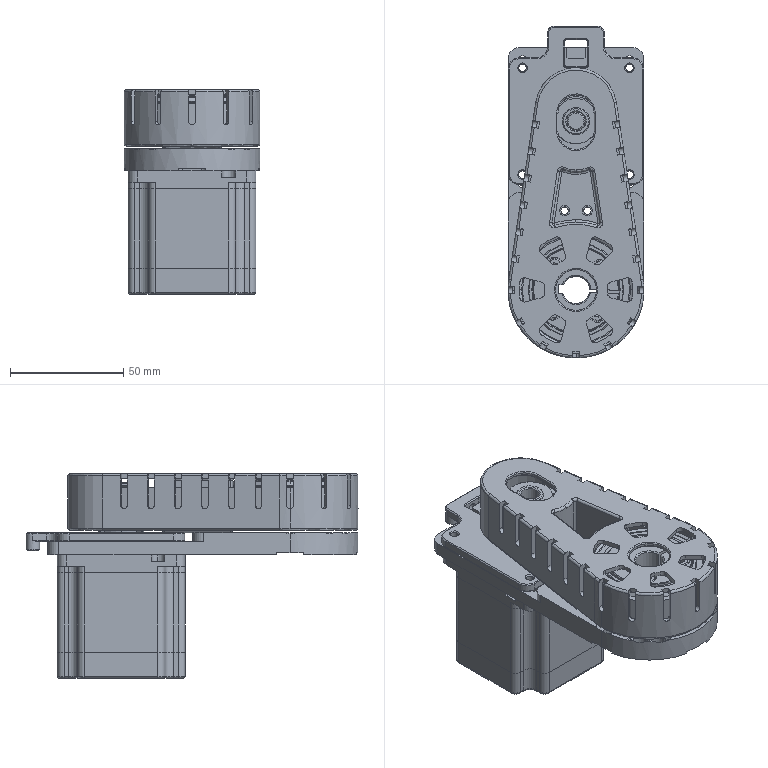Part | STEP file | Copy of CZ033-57 side link 3:1(60-60N)^K50A-1H20-S(formula driven)-L300-motor left- | 15 solids | 1292 faces | box 60 x 146.5 x 90.3 mm | volume 285335 mm3 | cylinder 717 | plane 329 | cone 142 | spline 91 | torus 13 | commonest cylinder face diameters 0.6 x170 1.82 x101 2 x64 47.96 x51 4 x40 6 x32